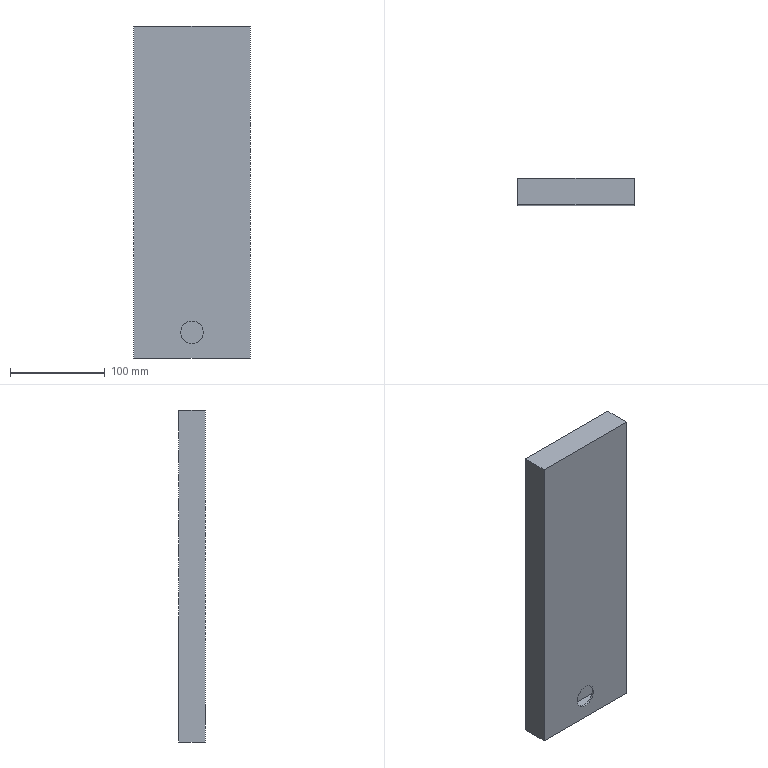Part | SolidWorks | features BaseBody 1, DelFace 1, ICE 1, MoveFace 1 | 1 solid | 140 faces | box 123 x 28 x 350 mm | volume 283122 mm3 | cylinder 128 | plane 12 | commonest cylinder face diameters 11.289 x126 24 x2